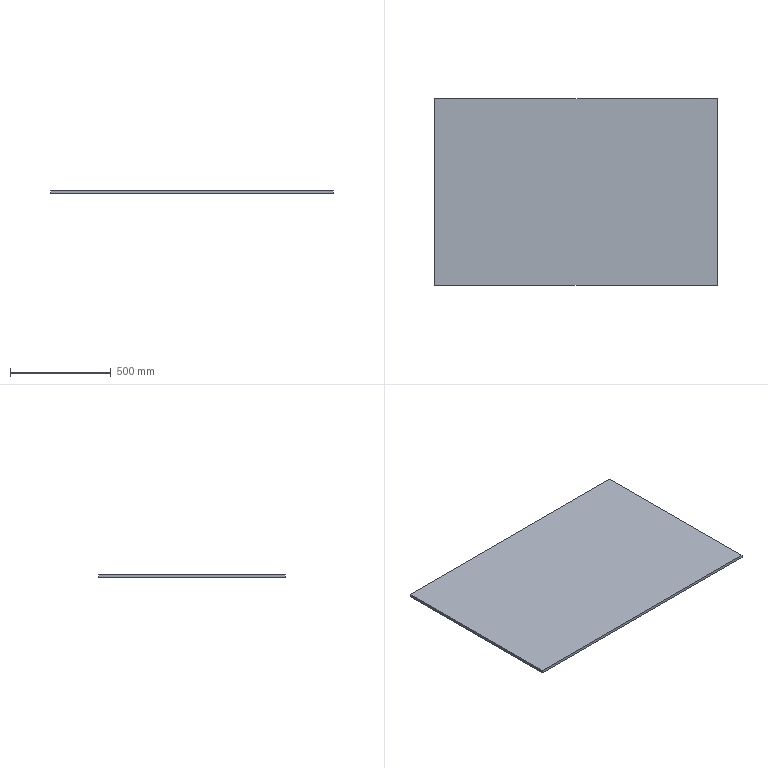Part | SolidWorks | features Extrusion 1 | 1 solid | 6 faces | box 1400 x 925 x 14 mm | volume 18130000 mm3 | plane 6
STEP:
#1=CARTESIAN_POINT('',(-775.,825.,0.));
#2=VERTEX_POINT('',#1);
#3=CARTESIAN_POINT('',(-775.,-100.,0.));
#4=VERTEX_POINT('',#3);
#5=CARTESIAN_POINT('',(-775.,825.,0.));
#6=DIRECTION('',(0.,-1.,0.));
#7=VECTOR('',#6,1000.);
#8=LINE('',#5,#7);
#9=EDGE_CURVE('',#2,#4,#8,.T.);
#10=ORIENTED_EDGE('',*,*,#9,.T.);
#11=CARTESIAN_POINT('',(-775.,-100.,14.));
#12=VERTEX_POINT('',#11);
#13=CARTESIAN_POINT('',(-775.,-100.,14.));
#14=DIRECTION('',(0.,0.,-1.));
#15=VECTOR('',#14,1000.);
#16=LINE('',#13,#15);
#17=EDGE_CURVE('',#12,#4,#16,.T.);
#18=ORIENTED_EDGE('',*,*,#17,.F.);
#19=CARTESIAN_POINT('',(-775.,825.,14.));
#20=VERTEX_POINT('',#19);
#21=CARTESIAN_POINT('',(-775.,825.,14.));
#22=DIRECTION('',(0.,-1.,0.));
#23=VECTOR('',#22,1000.);
#24=LINE('',#21,#23);
#25=EDGE_CURVE('',#20,#12,#24,.T.);
#26=ORIENTED_EDGE('',*,*,#25,.F.);
#27=CARTESIAN_POINT('',(-775.,825.,14.));
#28=DIRECTION('',(0.,0.,-1.));
#29=VECTOR('',#28,1000.);
#30=LINE('',#27,#29);
#31=EDGE_CURVE('',#20,#2,#30,.T.);
#32=ORIENTED_EDGE('',*,*,#31,.T.);
#33=EDGE_LOOP('',(#10,#18,#26,#32));
#34=FACE_OUTER_BOUND('',#33,.T.);
#35=CARTESIAN_POINT('',(-775.,825.,14.));
#36=DIRECTION('',(1.,0.,0.));
#37=DIRECTION('',(0.,1.,0.));
#38=AXIS2_PLACEMENT_3D('',#35,#36,#37);
#39=PLANE('',#38);
#40=ADVANCED_FACE('',(#34),#39,.F.);
#41=CARTESIAN_POINT('',(625.,-100.,0.));
#42=VERTEX_POINT('',#41);
#43=CARTESIAN_POINT('',(-775.,-100.,0.));
#44=DIRECTION('',(1.,0.,0.));
#45=VECTOR('',#44,1000.);
#46=LINE('',#43,#45);
#47=EDGE_CURVE('',#4,#42,#46,.T.);
#48=ORIENTED_EDGE('',*,*,#47,.T.);
#49=CARTESIAN_POINT('',(625.,-100.,14.));
#50=VERTEX_POINT('',#49);
#51=CARTESIAN_POINT('',(625.,-100.,14.));
#52=DIRECTION('',(0.,0.,-1.));
#53=VECTOR('',#52,1000.);
#54=LINE('',#51,#53);
#55=EDGE_CURVE('',#50,#42,#54,.T.);
#56=ORIENTED_EDGE('',*,*,#55,.F.);
#57=CARTESIAN_POINT('',(-775.,-100.,14.));
#58=DIRECTION('',(1.,0.,0.));
#59=VECTOR('',#58,1000.);
#60=LINE('',#57,#59);
#61=EDGE_CURVE('',#12,#50,#60,.T.);
#62=ORIENTED_EDGE('',*,*,#61,.F.);
#63=ORIENTED_EDGE('',*,*,#17,.T.);
#64=EDGE_LOOP('',(#48,#56,#62,#63));
#65=FACE_OUTER_BOUND('',#64,.T.);
#66=CARTESIAN_POINT('',(-775.,-100.,14.));
#67=DIRECTION('',(0.,1.,0.));
#68=DIRECTION('',(0.,0.,1.));
#69=AXIS2_PLACEMENT_3D('',#66,#67,#68);
#70=PLANE('',#69);
#71=ADVANCED_FACE('',(#65),#70,.F.);
#72=CARTESIAN_POINT('',(625.,825.,0.));
#73=VERTEX_POINT('',#72);
#74=CARTESIAN_POINT('',(625.,825.,0.));
#75=DIRECTION('',(0.,1.,0.));
#76=VECTOR('',#75,1000.);
#77=LINE('',#74,#76);
#78=EDGE_CURVE('',#42,#73,#77,.T.);
#79=ORIENTED_EDGE('',*,*,#78,.T.);
#80=CARTESIAN_POINT('',(625.,825.,14.));
#81=VERTEX_POINT('',#80);
#82=CARTESIAN_POINT('',(625.,825.,14.));
#83=DIRECTION('',(0.,0.,-1.));
#84=VECTOR('',#83,1000.);
#85=LINE('',#82,#84);
#86=EDGE_CURVE('',#81,#73,#85,.T.);
#87=ORIENTED_EDGE('',*,*,#86,.F.);
#88=CARTESIAN_POINT('',(625.,825.,14.));
#89=DIRECTION('',(0.,1.,0.));
#90=VECTOR('',#89,1000.);
#91=LINE('',#88,#90);
#92=EDGE_CURVE('',#50,#81,#91,.T.);
#93=ORIENTED_EDGE('',*,*,#92,.F.);
#94=ORIENTED_EDGE('',*,*,#55,.T.);
#95=EDGE_LOOP('',(#79,#87,#93,#94));
#96=FACE_OUTER_BOUND('',#95,.T.);
#97=CARTESIAN_POINT('',(625.,825.,14.));
#98=DIRECTION('',(-1.,0.,0.));
#99=DIRECTION('',(0.,-1.,0.));
#100=AXIS2_PLACEMENT_3D('',#97,#98,#99);
#101=PLANE('',#100);
#102=ADVANCED_FACE('',(#96),#101,.F.);
#103=CARTESIAN_POINT('',(-775.,825.,0.));
#104=DIRECTION('',(-1.,0.,0.));
#105=VECTOR('',#104,1000.);
#106=LINE('',#103,#105);
#107=EDGE_CURVE('',#73,#2,#106,.T.);
#108=ORIENTED_EDGE('',*,*,#107,.T.);
#109=ORIENTED_EDGE('',*,*,#31,.F.);
#110=CARTESIAN_POINT('',(-775.,825.,14.));
#111=DIRECTION('',(-1.,0.,0.));
#112=VECTOR('',#111,1000.);
#113=LINE('',#110,#112);
#114=EDGE_CURVE('',#81,#20,#113,.T.);
#115=ORIENTED_EDGE('',*,*,#114,.F.);
#116=ORIENTED_EDGE('',*,*,#86,.T.);
#117=EDGE_LOOP('',(#108,#109,#115,#116));
#118=FACE_OUTER_BOUND('',#117,.T.);
#119=CARTESIAN_POINT('',(-775.,825.,14.));
#120=DIRECTION('',(0.,-1.,0.));
#121=DIRECTION('',(0.,0.,-1.));
#122=AXIS2_PLACEMENT_3D('',#119,#120,#121);
#123=PLANE('',#122);
#124=ADVANCED_FACE('',(#118),#123,.F.);
#125=ORIENTED_EDGE('',*,*,#25,.T.);
#126=ORIENTED_EDGE('',*,*,#61,.T.);
#127=ORIENTED_EDGE('',*,*,#92,.T.);
#128=ORIENTED_EDGE('',*,*,#114,.T.);
#129=EDGE_LOOP('',(#125,#126,#127,#128));
#130=FACE_OUTER_BOUND('',#129,.T.);
#131=CARTESIAN_POINT('',(0.,0.,14.));
#132=DIRECTION('',(0.,0.,1.));
#133=DIRECTION('',(1.,0.,0.));
#134=AXIS2_PLACEMENT_3D('',#131,#132,#133);
#135=PLANE('',#134);
#136=ADVANCED_FACE('',(#130),#135,.T.);
#137=ORIENTED_EDGE('',*,*,#9,.F.);
#138=ORIENTED_EDGE('',*,*,#107,.F.);
#139=ORIENTED_EDGE('',*,*,#78,.F.);
#140=ORIENTED_EDGE('',*,*,#47,.F.);
#141=EDGE_LOOP('',(#137,#138,#139,#140));
#142=FACE_OUTER_BOUND('',#141,.T.);
#143=CARTESIAN_POINT('',(0.,0.,0.));
#144=DIRECTION('',(0.,0.,1.));
#145=DIRECTION('',(1.,0.,0.));
#146=AXIS2_PLACEMENT_3D('',#143,#144,#145);
#147=PLANE('',#146);
#148=ADVANCED_FACE('',(#142),#147,.F.);
#149=CLOSED_SHELL('',(#40,#71,#102,#124,#136,#148));
#150=MANIFOLD_SOLID_BREP('',#149);
#151=CARTESIAN_POINT('',(0.,0.,0.));
#152=DIRECTION('',(0.,0.,1.));
#153=DIRECTION('',(1.,0.,0.));
#154=AXIS2_PLACEMENT_3D('',#151,#152,#153);
#155=(LENGTH_UNIT()NAMED_UNIT(*)SI_UNIT(.MILLI.,.METRE.));
#156=UNCERTAINTY_MEASURE_WITH_UNIT(LENGTH_MEASURE(0.00001),#155,'','');
#157=(NAMED_UNIT(*)PLANE_ANGLE_UNIT()SI_UNIT($,.RADIAN.));
#158=(NAMED_UNIT(*)SI_UNIT($,.STERADIAN.)SOLID_ANGLE_UNIT());
#159=(GEOMETRIC_REPRESENTATION_CONTEXT(3)GLOBAL_UNCERTAINTY_ASSIGNED_CONTEXT((#156))GLOBAL_UNIT_ASSIGNED_CONTEXT((#155,#157,#158))REPRESENTATION_CONTEXT('',''));
#160=ADVANCED_BREP_SHAPE_REPRESENTATION('',(#150,#154),#159);